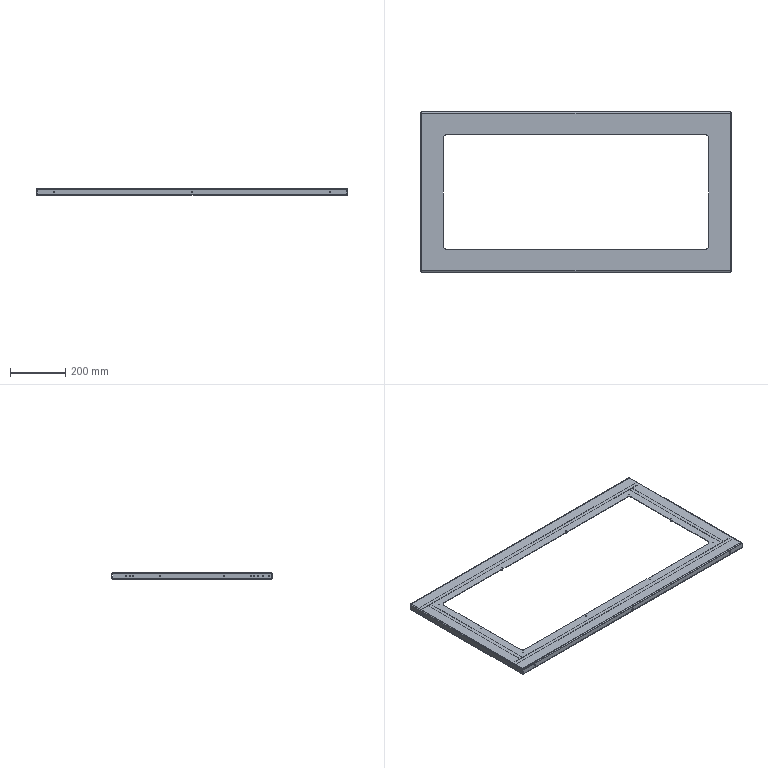Part | NX | features BREP 5 | 5 solids | 262 faces | box 1126 x 580 x 25 mm | volume 933574 mm3 | plane 124 | cylinder 102 | cone 20 | spline 16 | commonest cylinder face diameters 4.2 x24 5 x20 3.3 x16 4 x16 7 x8 8 x8